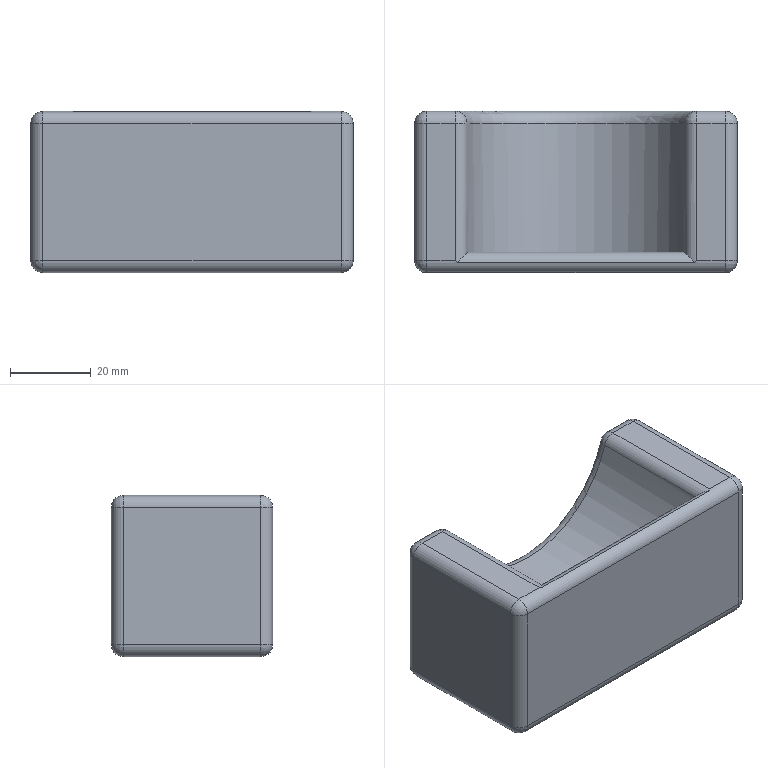Part | SolidWorks | features Extrusion 1, Fillet 1, ICE 1 | 1 solid | 36 faces | box 80 x 40 x 40 mm | volume 93219 mm3 | cylinder 17 | sphere 10 | plane 8 | torus 1 | commonest cylinder face diameters 6 x16 56 x1
STEP:
#1=CARTESIAN_POINT('',(29.95,3.,20.));
#2=VERTEX_POINT('',#1);
#3=CARTESIAN_POINT('',(37.,3.,20.));
#4=VERTEX_POINT('',#3);
#5=CARTESIAN_POINT('',(-40.,3.,20.));
#6=DIRECTION('',(1.,0.,0.));
#7=VECTOR('',#6,1000.);
#8=LINE('',#5,#7);
#9=EDGE_CURVE('',#2,#4,#8,.T.);
#10=ORIENTED_EDGE('',*,*,#9,.T.);
#11=CARTESIAN_POINT('',(37.,37.,20.));
#12=VERTEX_POINT('',#11);
#13=CARTESIAN_POINT('',(37.,40.,20.));
#14=DIRECTION('',(0.,1.,0.));
#15=VECTOR('',#14,1000.);
#16=LINE('',#13,#15);
#17=EDGE_CURVE('',#4,#12,#16,.T.);
#18=ORIENTED_EDGE('',*,*,#17,.T.);
#19=CARTESIAN_POINT('',(29.95,37.,20.));
#20=VERTEX_POINT('',#19);
#21=CARTESIAN_POINT('',(27.55,37.,20.));
#22=DIRECTION('',(-1.,0.,0.));
#23=VECTOR('',#22,1000.);
#24=LINE('',#21,#23);
#25=EDGE_CURVE('',#12,#20,#24,.T.);
#26=ORIENTED_EDGE('',*,*,#25,.T.);
#27=CARTESIAN_POINT('',(29.95,40.,20.));
#28=DIRECTION('',(0.,-1.,0.));
#29=VECTOR('',#28,1000.);
#30=LINE('',#27,#29);
#31=EDGE_CURVE('',#20,#2,#30,.T.);
#32=ORIENTED_EDGE('',*,*,#31,.T.);
#33=EDGE_LOOP('',(#10,#18,#26,#32));
#34=FACE_OUTER_BOUND('',#33,.T.);
#35=CARTESIAN_POINT('',(-40.,40.,20.));
#36=DIRECTION('',(0.,0.,-1.));
#37=DIRECTION('',(-1.,0.,0.));
#38=AXIS2_PLACEMENT_3D('',#35,#36,#37);
#39=PLANE('',#38);
#40=ADVANCED_FACE('',(#34),#39,.F.);
#41=CARTESIAN_POINT('',(40.,3.,-17.));
#42=VERTEX_POINT('',#41);
#43=CARTESIAN_POINT('',(40.,37.,-17.));
#44=VERTEX_POINT('',#43);
#45=CARTESIAN_POINT('',(40.,40.,-17.));
#46=DIRECTION('',(0.,1.,0.));
#47=VECTOR('',#46,1000.);
#48=LINE('',#45,#47);
#49=EDGE_CURVE('',#42,#44,#48,.T.);
#50=ORIENTED_EDGE('',*,*,#49,.T.);
#51=CARTESIAN_POINT('',(40.,37.,17.));
#52=VERTEX_POINT('',#51);
#53=CARTESIAN_POINT('',(40.,37.,20.));
#54=DIRECTION('',(0.,0.,1.));
#55=VECTOR('',#54,1000.);
#56=LINE('',#53,#55);
#57=EDGE_CURVE('',#44,#52,#56,.T.);
#58=ORIENTED_EDGE('',*,*,#57,.T.);
#59=CARTESIAN_POINT('',(40.,3.,17.));
#60=VERTEX_POINT('',#59);
#61=CARTESIAN_POINT('',(40.,40.,17.));
#62=DIRECTION('',(0.,-1.,0.));
#63=VECTOR('',#62,1000.);
#64=LINE('',#61,#63);
#65=EDGE_CURVE('',#52,#60,#64,.T.);
#66=ORIENTED_EDGE('',*,*,#65,.T.);
#67=CARTESIAN_POINT('',(40.,3.,-20.));
#68=DIRECTION('',(0.,0.,-1.));
#69=VECTOR('',#68,1000.);
#70=LINE('',#67,#69);
#71=EDGE_CURVE('',#60,#42,#70,.T.);
#72=ORIENTED_EDGE('',*,*,#71,.T.);
#73=EDGE_LOOP('',(#50,#58,#66,#72));
#74=FACE_OUTER_BOUND('',#73,.T.);
#75=CARTESIAN_POINT('',(40.,40.,-20.));
#76=DIRECTION('',(-1.,0.,0.));
#77=DIRECTION('',(0.,0.,1.));
#78=AXIS2_PLACEMENT_3D('',#75,#76,#77);
#79=PLANE('',#78);
#80=ADVANCED_FACE('',(#74),#79,.F.);
#81=CARTESIAN_POINT('',(-37.,37.,-20.));
#82=VERTEX_POINT('',#81);
#83=CARTESIAN_POINT('',(37.,37.,-20.));
#84=VERTEX_POINT('',#83);
#85=CARTESIAN_POINT('',(40.,37.,-20.));
#86=DIRECTION('',(1.,0.,0.));
#87=VECTOR('',#86,1000.);
#88=LINE('',#85,#87);
#89=EDGE_CURVE('',#82,#84,#88,.T.);
#90=ORIENTED_EDGE('',*,*,#89,.T.);
#91=CARTESIAN_POINT('',(37.,3.,-20.));
#92=VERTEX_POINT('',#91);
#93=CARTESIAN_POINT('',(37.,40.,-20.));
#94=DIRECTION('',(0.,-1.,0.));
#95=VECTOR('',#94,1000.);
#96=LINE('',#93,#95);
#97=EDGE_CURVE('',#84,#92,#96,.T.);
#98=ORIENTED_EDGE('',*,*,#97,.T.);
#99=CARTESIAN_POINT('',(-37.,3.,-20.));
#100=VERTEX_POINT('',#99);
#101=CARTESIAN_POINT('',(-40.,3.,-20.));
#102=DIRECTION('',(-1.,0.,0.));
#103=VECTOR('',#102,1000.);
#104=LINE('',#101,#103);
#105=EDGE_CURVE('',#92,#100,#104,.T.);
#106=ORIENTED_EDGE('',*,*,#105,.T.);
#107=CARTESIAN_POINT('',(-37.,40.,-20.));
#108=DIRECTION('',(0.,1.,0.));
#109=VECTOR('',#108,1000.);
#110=LINE('',#107,#109);
#111=EDGE_CURVE('',#100,#82,#110,.T.);
#112=ORIENTED_EDGE('',*,*,#111,.T.);
#113=EDGE_LOOP('',(#90,#98,#106,#112));
#114=FACE_OUTER_BOUND('',#113,.T.);
#115=CARTESIAN_POINT('',(-40.,40.,-20.));
#116=DIRECTION('',(0.,0.,1.));
#117=DIRECTION('',(1.,0.,0.));
#118=AXIS2_PLACEMENT_3D('',#115,#116,#117);
#119=PLANE('',#118);
#120=ADVANCED_FACE('',(#114),#119,.F.);
#121=CARTESIAN_POINT('',(-40.,37.,17.));
#122=VERTEX_POINT('',#121);
#123=CARTESIAN_POINT('',(-40.,37.,-17.));
#124=VERTEX_POINT('',#123);
#125=CARTESIAN_POINT('',(-40.,37.,-20.));
#126=DIRECTION('',(0.,0.,-1.));
#127=VECTOR('',#126,1000.);
#128=LINE('',#125,#127);
#129=EDGE_CURVE('',#122,#124,#128,.T.);
#130=ORIENTED_EDGE('',*,*,#129,.T.);
#131=CARTESIAN_POINT('',(-40.,3.,-17.));
#132=VERTEX_POINT('',#131);
#133=CARTESIAN_POINT('',(-40.,40.,-17.));
#134=DIRECTION('',(0.,-1.,0.));
#135=VECTOR('',#134,1000.);
#136=LINE('',#133,#135);
#137=EDGE_CURVE('',#124,#132,#136,.T.);
#138=ORIENTED_EDGE('',*,*,#137,.T.);
#139=CARTESIAN_POINT('',(-40.,3.,17.));
#140=VERTEX_POINT('',#139);
#141=CARTESIAN_POINT('',(-40.,3.,-20.));
#142=DIRECTION('',(0.,0.,1.));
#143=VECTOR('',#142,1000.);
#144=LINE('',#141,#143);
#145=EDGE_CURVE('',#132,#140,#144,.T.);
#146=ORIENTED_EDGE('',*,*,#145,.T.);
#147=CARTESIAN_POINT('',(-40.,40.,17.));
#148=DIRECTION('',(0.,1.,0.));
#149=VECTOR('',#148,1000.);
#150=LINE('',#147,#149);
#151=EDGE_CURVE('',#140,#122,#150,.T.);
#152=ORIENTED_EDGE('',*,*,#151,.T.);
#153=EDGE_LOOP('',(#130,#138,#146,#152));
#154=FACE_OUTER_BOUND('',#153,.T.);
#155=CARTESIAN_POINT('',(-40.,40.,-20.));
#156=DIRECTION('',(1.,0.,0.));
#157=DIRECTION('',(0.,0.,-1.));
#158=AXIS2_PLACEMENT_3D('',#155,#156,#157);
#159=PLANE('',#158);
#160=ADVANCED_FACE('',(#154),#159,.F.);
#161=CARTESIAN_POINT('',(-29.95,3.,20.));
#162=VERTEX_POINT('',#161);
#163=CARTESIAN_POINT('',(-29.95,37.,20.));
#164=VERTEX_POINT('',#163);
#165=CARTESIAN_POINT('',(-29.95,40.,20.));
#166=DIRECTION('',(0.,1.,0.));
#167=VECTOR('',#166,1000.);
#168=LINE('',#165,#167);
#169=EDGE_CURVE('',#162,#164,#168,.T.);
#170=ORIENTED_EDGE('',*,*,#169,.T.);
#171=CARTESIAN_POINT('',(-37.,37.,20.));
#172=VERTEX_POINT('',#171);
#173=CARTESIAN_POINT('',(-40.,37.,20.));
#174=DIRECTION('',(-1.,0.,0.));
#175=VECTOR('',#174,1000.);
#176=LINE('',#173,#175);
#177=EDGE_CURVE('',#164,#172,#176,.T.);
#178=ORIENTED_EDGE('',*,*,#177,.T.);
#179=CARTESIAN_POINT('',(-37.,3.,20.));
#180=VERTEX_POINT('',#179);
#181=CARTESIAN_POINT('',(-37.,40.,20.));
#182=DIRECTION('',(0.,-1.,0.));
#183=VECTOR('',#182,1000.);
#184=LINE('',#181,#183);
#185=EDGE_CURVE('',#172,#180,#184,.T.);
#186=ORIENTED_EDGE('',*,*,#185,.T.);
#187=CARTESIAN_POINT('',(-40.,3.,20.));
#188=DIRECTION('',(1.,0.,0.));
#189=VECTOR('',#188,1000.);
#190=LINE('',#187,#189);
#191=EDGE_CURVE('',#180,#162,#190,.T.);
#192=ORIENTED_EDGE('',*,*,#191,.T.);
#193=EDGE_LOOP('',(#170,#178,#186,#192));
#194=FACE_OUTER_BOUND('',#193,.T.);
#195=CARTESIAN_POINT('',(-40.,40.,20.));
#196=DIRECTION('',(0.,0.,-1.));
#197=DIRECTION('',(-1.,0.,0.));
#198=AXIS2_PLACEMENT_3D('',#195,#196,#197);
#199=PLANE('',#198);
#200=ADVANCED_FACE('',(#194),#199,.F.);
#201=CARTESIAN_POINT('',(-29.95,40.,17.));
#202=VERTEX_POINT('',#201);
#203=CARTESIAN_POINT('',(29.95,40.,17.));
#204=VERTEX_POINT('',#203);
#205=CARTESIAN_POINT('',(0.,40.,25.));
#206=DIRECTION('',(0.,-1.,0.));
#207=DIRECTION('',(0.,0.,1.));
#208=AXIS2_PLACEMENT_3D('',#205,#206,#207);
#209=CIRCLE('',#208,31.);
#210=EDGE_CURVE('',#202,#204,#209,.T.);
#211=ORIENTED_EDGE('',*,*,#210,.T.);
#212=CARTESIAN_POINT('',(37.,40.,17.));
#213=VERTEX_POINT('',#212);
#214=CARTESIAN_POINT('',(40.,40.,17.));
#215=DIRECTION('',(1.,0.,0.));
#216=VECTOR('',#215,1000.);
#217=LINE('',#214,#216);
#218=EDGE_CURVE('',#204,#213,#217,.T.);
#219=ORIENTED_EDGE('',*,*,#218,.T.);
#220=CARTESIAN_POINT('',(37.,40.,-17.));
#221=VERTEX_POINT('',#220);
#222=CARTESIAN_POINT('',(37.,40.,-20.));
#223=DIRECTION('',(0.,0.,-1.));
#224=VECTOR('',#223,1000.);
#225=LINE('',#222,#224);
#226=EDGE_CURVE('',#213,#221,#225,.T.);
#227=ORIENTED_EDGE('',*,*,#226,.T.);
#228=CARTESIAN_POINT('',(-37.,40.,-17.));
#229=VERTEX_POINT('',#228);
#230=CARTESIAN_POINT('',(-40.,40.,-17.));
#231=DIRECTION('',(-1.,0.,0.));
#232=VECTOR('',#231,1000.);
#233=LINE('',#230,#232);
#234=EDGE_CURVE('',#221,#229,#233,.T.);
#235=ORIENTED_EDGE('',*,*,#234,.T.);
#236=CARTESIAN_POINT('',(-37.,40.,17.));
#237=VERTEX_POINT('',#236);
#238=CARTESIAN_POINT('',(-37.,40.,20.));
#239=DIRECTION('',(0.,0.,1.));
#240=VECTOR('',#239,1000.);
#241=LINE('',#238,#240);
#242=EDGE_CURVE('',#229,#237,#241,.T.);
#243=ORIENTED_EDGE('',*,*,#242,.T.);
#244=CARTESIAN_POINT('',(-27.55,40.,17.));
#245=DIRECTION('',(1.,0.,0.));
#246=VECTOR('',#245,1000.);
#247=LINE('',#244,#246);
#248=EDGE_CURVE('',#237,#202,#247,.T.);
#249=ORIENTED_EDGE('',*,*,#248,.T.);
#250=EDGE_LOOP('',(#211,#219,#227,#235,#243,#249));
#251=FACE_OUTER_BOUND('',#250,.T.);
#252=CARTESIAN_POINT('',(0.,40.,0.));
#253=DIRECTION('',(0.,1.,0.));
#254=DIRECTION('',(0.,0.,1.));
#255=AXIS2_PLACEMENT_3D('',#252,#253,#254);
#256=PLANE('',#255);
#257=ADVANCED_FACE('',(#251),#256,.T.);
#258=CARTESIAN_POINT('',(-37.,0.,17.));
#259=VERTEX_POINT('',#258);
#260=CARTESIAN_POINT('',(-37.,0.,-17.));
#261=VERTEX_POINT('',#260);
#262=CARTESIAN_POINT('',(-37.,0.,0.));
#263=DIRECTION('',(0.,0.,-1.));
#264=VECTOR('',#263,1000.);
#265=LINE('',#262,#264);
#266=EDGE_CURVE('',#259,#261,#265,.T.);
#267=ORIENTED_EDGE('',*,*,#266,.T.);
#268=CARTESIAN_POINT('',(37.,0.,-17.));
#269=VERTEX_POINT('',#268);
#270=CARTESIAN_POINT('',(0.,0.,-17.));
#271=DIRECTION('',(1.,0.,0.));
#272=VECTOR('',#271,1000.);
#273=LINE('',#270,#272);
#274=EDGE_CURVE('',#261,#269,#273,.T.);
#275=ORIENTED_EDGE('',*,*,#274,.T.);
#276=CARTESIAN_POINT('',(37.,0.,17.));
#277=VERTEX_POINT('',#276);
#278=CARTESIAN_POINT('',(37.,0.,0.));
#279=DIRECTION('',(0.,0.,1.));
#280=VECTOR('',#279,1000.);
#281=LINE('',#278,#280);
#282=EDGE_CURVE('',#269,#277,#281,.T.);
#283=ORIENTED_EDGE('',*,*,#282,.T.);
#284=CARTESIAN_POINT('',(0.,0.,17.));
#285=DIRECTION('',(-1.,0.,0.));
#286=VECTOR('',#285,1000.);
#287=LINE('',#284,#286);
#288=EDGE_CURVE('',#277,#259,#287,.T.);
#289=ORIENTED_EDGE('',*,*,#288,.T.);
#290=EDGE_LOOP('',(#267,#275,#283,#289));
#291=FACE_OUTER_BOUND('',#290,.T.);
#292=CARTESIAN_POINT('',(0.,0.,0.));
#293=DIRECTION('',(0.,1.,0.));
#294=DIRECTION('',(0.,0.,1.));
#295=AXIS2_PLACEMENT_3D('',#292,#293,#294);
#296=PLANE('',#295);
#297=ADVANCED_FACE('',(#291),#296,.F.);
#298=CARTESIAN_POINT('',(26.833,5.,17.));
#299=VERTEX_POINT('',#298);
#300=CARTESIAN_POINT('',(-26.833,5.,17.));
#301=VERTEX_POINT('',#300);
#302=CARTESIAN_POINT('',(0.,5.,25.));
#303=DIRECTION('',(0.,1.,0.));
#304=DIRECTION('',(0.,0.,1.));
#305=AXIS2_PLACEMENT_3D('',#302,#303,#304);
#306=CIRCLE('',#305,28.);
#307=EDGE_CURVE('',#299,#301,#306,.T.);
#308=ORIENTED_EDGE('',*,*,#307,.T.);
#309=CARTESIAN_POINT('',(27.55,5.,17.));
#310=DIRECTION('',(1.,0.,0.));
#311=VECTOR('',#310,1000.);
#312=LINE('',#309,#311);
#313=EDGE_CURVE('',#301,#299,#312,.T.);
#314=ORIENTED_EDGE('',*,*,#313,.T.);
#315=EDGE_LOOP('',(#308,#314));
#316=FACE_OUTER_BOUND('',#315,.T.);
#317=CARTESIAN_POINT('',(0.,5.,25.));
#318=DIRECTION('',(0.,1.,0.));
#319=DIRECTION('',(0.,0.,1.));
#320=AXIS2_PLACEMENT_3D('',#317,#318,#319);
#321=PLANE('',#320);
#322=ADVANCED_FACE('',(#316),#321,.T.);
#323=ORIENTED_EDGE('',*,*,#307,.F.);
#324=CARTESIAN_POINT('',(27.052,4.898,17.774));
#325=VERTEX_POINT('',#324);
#326=CARTESIAN_POINT('',(26.833,5.,17.));
#327=CARTESIAN_POINT('',(26.911,5.,17.261));
#328=CARTESIAN_POINT('',(26.983,4.966,17.519));
#329=CARTESIAN_POINT('',(27.052,4.898,17.774));
#330=B_SPLINE_CURVE_WITH_KNOTS('',3,(#326,#327,#328,#329),.UNSPECIFIED.,.F.,.F.,(4,4),(0.,0.0008109),.UNSPECIFIED.);
#331=EDGE_CURVE('',#299,#325,#330,.T.);
#332=ORIENTED_EDGE('',*,*,#331,.T.);
#333=CARTESIAN_POINT('',(27.052,37.,17.774));
#334=VERTEX_POINT('',#333);
#335=CARTESIAN_POINT('',(27.052,5.,17.774));
#336=DIRECTION('',(0.,1.,0.));
#337=VECTOR('',#336,1000.);
#338=LINE('',#335,#337);
#339=EDGE_CURVE('',#325,#334,#338,.T.);
#340=ORIENTED_EDGE('',*,*,#339,.T.);
#341=CARTESIAN_POINT('',(-27.052,37.,17.774));
#342=VERTEX_POINT('',#341);
#343=CARTESIAN_POINT('',(0.,37.,25.));
#344=DIRECTION('',(0.,1.,0.));
#345=DIRECTION('',(0.,0.,1.));
#346=AXIS2_PLACEMENT_3D('',#343,#344,#345);
#347=CIRCLE('',#346,28.);
#348=EDGE_CURVE('',#334,#342,#347,.T.);
#349=ORIENTED_EDGE('',*,*,#348,.T.);
#350=CARTESIAN_POINT('',(-27.052,4.898,17.774));
#351=VERTEX_POINT('',#350);
#352=CARTESIAN_POINT('',(-27.052,5.,17.774));
#353=DIRECTION('',(0.,-1.,0.));
#354=VECTOR('',#353,1000.);
#355=LINE('',#352,#354);
#356=EDGE_CURVE('',#342,#351,#355,.T.);
#357=ORIENTED_EDGE('',*,*,#356,.T.);
#358=CARTESIAN_POINT('',(-27.052,4.898,17.774));
#359=CARTESIAN_POINT('',(-26.983,4.966,17.519));
#360=CARTESIAN_POINT('',(-26.911,5.,17.261));
#361=CARTESIAN_POINT('',(-26.833,5.,17.));
#362=B_SPLINE_CURVE_WITH_KNOTS('',3,(#358,#359,#360,#361),.UNSPECIFIED.,.F.,.F.,(4,4),(0.,0.0008109),.UNSPECIFIED.);
#363=EDGE_CURVE('',#351,#301,#362,.T.);
#364=ORIENTED_EDGE('',*,*,#363,.T.);
#365=EDGE_LOOP('',(#323,#332,#340,#349,#357,#364));
#366=FACE_OUTER_BOUND('',#365,.T.);
#367=CARTESIAN_POINT('',(0.,5.,25.));
#368=DIRECTION('',(0.,1.,0.));
#369=DIRECTION('',(0.,0.,1.));
#370=AXIS2_PLACEMENT_3D('',#367,#368,#369);
#371=CYLINDRICAL_SURFACE('',#370,28.);
#372=ADVANCED_FACE('',(#366),#371,.F.);
#373=CARTESIAN_POINT('',(-37.,3.,-17.));
#374=DIRECTION('',(-1.,0.,0.));
#375=DIRECTION('',(0.,0.,1.));
#376=AXIS2_PLACEMENT_3D('',#373,#374,#375);
#377=CIRCLE('',#376,3.);
#378=EDGE_CURVE('',#100,#261,#377,.T.);
#379=ORIENTED_EDGE('',*,*,#378,.F.);
#380=ORIENTED_EDGE('',*,*,#105,.F.);
#381=CARTESIAN_POINT('',(37.,3.,-17.));
#382=DIRECTION('',(1.,0.,0.));
#383=DIRECTION('',(0.,0.,-1.));
#384=AXIS2_PLACEMENT_3D('',#381,#382,#383);
#385=CIRCLE('',#384,3.);
#386=EDGE_CURVE('',#269,#92,#385,.T.);
#387=ORIENTED_EDGE('',*,*,#386,.F.);
#388=ORIENTED_EDGE('',*,*,#274,.F.);
#389=EDGE_LOOP('',(#379,#380,#387,#388));
#390=FACE_OUTER_BOUND('',#389,.T.);
#391=CARTESIAN_POINT('',(-40.,3.,-17.));
#392=DIRECTION('',(-1.,0.,0.));
#393=DIRECTION('',(0.,0.,1.));
#394=AXIS2_PLACEMENT_3D('',#391,#392,#393);
#395=CYLINDRICAL_SURFACE('',#394,3.);
#396=ADVANCED_FACE('',(#390),#395,.T.);
#397=CARTESIAN_POINT('',(37.,37.,-17.));
#398=DIRECTION('',(0.,1.,0.));
#399=DIRECTION('',(0.,0.,1.));
#400=AXIS2_PLACEMENT_3D('',#397,#398,#399);
#401=CIRCLE('',#400,3.);
#402=EDGE_CURVE('',#44,#84,#401,.T.);
#403=ORIENTED_EDGE('',*,*,#402,.F.);
#404=ORIENTED_EDGE('',*,*,#49,.F.);
#405=CARTESIAN_POINT('',(37.,3.,-17.));
#406=DIRECTION('',(0.,-1.,0.));
#407=DIRECTION('',(0.,0.,-1.));
#408=AXIS2_PLACEMENT_3D('',#405,#406,#407);
#409=CIRCLE('',#408,3.);
#410=EDGE_CURVE('',#92,#42,#409,.T.);
#411=ORIENTED_EDGE('',*,*,#410,.F.);
#412=ORIENTED_EDGE('',*,*,#97,.F.);
#413=EDGE_LOOP('',(#403,#404,#411,#412));
#414=FACE_OUTER_BOUND('',#413,.T.);
#415=CARTESIAN_POINT('',(37.,40.,-17.));
#416=DIRECTION('',(0.,-1.,0.));
#417=DIRECTION('',(0.,0.,-1.));
#418=AXIS2_PLACEMENT_3D('',#415,#416,#417);
#419=CYLINDRICAL_SURFACE('',#418,3.);
#420=ADVANCED_FACE('',(#414),#419,.T.);
#421=CARTESIAN_POINT('',(37.,37.,17.));
#422=DIRECTION('',(0.,0.,1.));
#423=DIRECTION('',(0.,-1.,0.));
#424=AXIS2_PLACEMENT_3D('',#421,#422,#423);
#425=CIRCLE('',#424,3.);
#426=EDGE_CURVE('',#52,#213,#425,.T.);
#427=ORIENTED_EDGE('',*,*,#426,.F.);
#428=ORIENTED_EDGE('',*,*,#57,.F.);
#429=CARTESIAN_POINT('',(37.,37.,-17.));
#430=DIRECTION('',(0.,0.,-1.));
#431=DIRECTION('',(-1.,0.,0.));
#432=AXIS2_PLACEMENT_3D('',#429,#430,#431);
#433=CIRCLE('',#432,3.);
#434=EDGE_CURVE('',#221,#44,#433,.T.);
#435=ORIENTED_EDGE('',*,*,#434,.F.);
#436=ORIENTED_EDGE('',*,*,#226,.F.);
#437=EDGE_LOOP('',(#427,#428,#435,#436));
#438=FACE_OUTER_BOUND('',#437,.T.);
#439=CARTESIAN_POINT('',(37.,37.,0.));
#440=DIRECTION('',(0.,0.,1.));
#441=DIRECTION('',(1.,0.,0.));
#442=AXIS2_PLACEMENT_3D('',#439,#440,#441);
#443=CYLINDRICAL_SURFACE('',#442,3.);
#444=ADVANCED_FACE('',(#438),#443,.T.);
#445=ORIENTED_EDGE('',*,*,#386,.T.);
#446=ORIENTED_EDGE('',*,*,#410,.T.);
#447=CARTESIAN_POINT('',(37.,3.,-17.));
#448=DIRECTION('',(0.,0.,1.));
#449=DIRECTION('',(-1.,0.,0.));
#450=AXIS2_PLACEMENT_3D('',#447,#448,#449);
#451=CIRCLE('',#450,3.);
#452=EDGE_CURVE('',#269,#42,#451,.T.);
#453=ORIENTED_EDGE('',*,*,#452,.F.);
#454=EDGE_LOOP('',(#445,#446,#453));
#455=FACE_OUTER_BOUND('',#454,.T.);
#456=CARTESIAN_POINT('',(37.,3.,-17.));
#457=DIRECTION('',(0.,1.,0.));
#458=DIRECTION('',(1.,0.,0.));
#459=AXIS2_PLACEMENT_3D('',#456,#457,#458);
#460=SPHERICAL_SURFACE('',#459,3.);
#461=ADVANCED_FACE('',(#455),#460,.T.);
#462=CARTESIAN_POINT('',(-37.,3.,-17.));
#463=DIRECTION('',(0.,1.,0.));
#464=DIRECTION('',(0.,0.,-1.));
#465=AXIS2_PLACEMENT_3D('',#462,#463,#464);
#466=CIRCLE('',#465,3.);
#467=EDGE_CURVE('',#100,#132,#466,.T.);
#468=ORIENTED_EDGE('',*,*,#467,.F.);
#469=ORIENTED_EDGE('',*,*,#378,.T.);
#470=CARTESIAN_POINT('',(-37.,3.,-17.));
#471=DIRECTION('',(0.,0.,1.));
#472=DIRECTION('',(-1.,0.,0.));
#473=AXIS2_PLACEMENT_3D('',#470,#471,#472);
#474=CIRCLE('',#473,3.);
#475=EDGE_CURVE('',#132,#261,#474,.T.);
#476=ORIENTED_EDGE('',*,*,#475,.F.);
#477=EDGE_LOOP('',(#468,#469,#476));
#478=FACE_OUTER_BOUND('',#477,.T.);
#479=CARTESIAN_POINT('',(-37.,3.,-17.));
#480=DIRECTION('',(0.,1.,0.));
#481=DIRECTION('',(1.,0.,0.));
#482=AXIS2_PLACEMENT_3D('',#479,#480,#481);
#483=SPHERICAL_SURFACE('',#482,3.);
#484=ADVANCED_FACE('',(#478),#483,.T.);
#485=ORIENTED_EDGE('',*,*,#434,.T.);
#486=ORIENTED_EDGE('',*,*,#402,.T.);
#487=CARTESIAN_POINT('',(37.,37.,-17.));
#488=DIRECTION('',(-1.,0.,0.));
#489=DIRECTION('',(0.,0.,-1.));
#490=AXIS2_PLACEMENT_3D('',#487,#488,#489);
#491=CIRCLE('',#490,3.);
#492=EDGE_CURVE('',#221,#84,#491,.T.);
#493=ORIENTED_EDGE('',*,*,#492,.F.);
#494=EDGE_LOOP('',(#485,#486,#493));
#495=FACE_OUTER_BOUND('',#494,.T.);
#496=CARTESIAN_POINT('',(37.,37.,-17.));
#497=DIRECTION('',(0.,1.,0.));
#498=DIRECTION('',(1.,0.,0.));
#499=AXIS2_PLACEMENT_3D('',#496,#497,#498);
#500=SPHERICAL_SURFACE('',#499,3.);
#501=ADVANCED_FACE('',(#495),#500,.T.);
#502=CARTESIAN_POINT('',(37.,37.,17.));
#503=DIRECTION('',(-1.,0.,0.));
#504=DIRECTION('',(0.,0.,-1.));
#505=AXIS2_PLACEMENT_3D('',#502,#503,#504);
#506=CIRCLE('',#505,3.);
#507=EDGE_CURVE('',#12,#213,#506,.T.);
#508=ORIENTED_EDGE('',*,*,#507,.F.);
#509=CARTESIAN_POINT('',(37.,37.,17.));
#510=DIRECTION('',(0.,-1.,0.));
#511=DIRECTION('',(0.,0.,1.));
#512=AXIS2_PLACEMENT_3D('',#509,#510,#511);
#513=CIRCLE('',#512,3.);
#514=EDGE_CURVE('',#52,#12,#513,.T.);
#515=ORIENTED_EDGE('',*,*,#514,.F.);
#516=ORIENTED_EDGE('',*,*,#426,.T.);
#517=EDGE_LOOP('',(#508,#515,#516));
#518=FACE_OUTER_BOUND('',#517,.T.);
#519=CARTESIAN_POINT('',(37.,37.,17.));
#520=DIRECTION('',(0.,1.,0.));
#521=DIRECTION('',(1.,0.,0.));
#522=AXIS2_PLACEMENT_3D('',#519,#520,#521);
#523=SPHERICAL_SURFACE('',#522,3.);
#524=ADVANCED_FACE('',(#518),#523,.T.);
#525=ORIENTED_EDGE('',*,*,#514,.T.);
#526=ORIENTED_EDGE('',*,*,#17,.F.);
#527=CARTESIAN_POINT('',(37.,3.,17.));
#528=DIRECTION('',(0.,-1.,0.));
#529=DIRECTION('',(0.,0.,-1.));
#530=AXIS2_PLACEMENT_3D('',#527,#528,#529);
#531=CIRCLE('',#530,3.);
#532=EDGE_CURVE('',#60,#4,#531,.T.);
#533=ORIENTED_EDGE('',*,*,#532,.F.);
#534=ORIENTED_EDGE('',*,*,#65,.F.);
#535=EDGE_LOOP('',(#525,#526,#533,#534));
#536=FACE_OUTER_BOUND('',#535,.T.);
#537=CARTESIAN_POINT('',(37.,40.,17.));
#538=DIRECTION('',(0.,-1.,0.));
#539=DIRECTION('',(0.,0.,-1.));
#540=AXIS2_PLACEMENT_3D('',#537,#538,#539);
#541=CYLINDRICAL_SURFACE('',#540,3.);
#542=ADVANCED_FACE('',(#536),#541,.T.);
#543=ORIENTED_EDGE('',*,*,#452,.T.);
#544=ORIENTED_EDGE('',*,*,#71,.F.);
#545=CARTESIAN_POINT('',(37.,3.,17.));
#546=DIRECTION('',(0.,0.,1.));
#547=DIRECTION('',(1.,0.,0.));
#548=AXIS2_PLACEMENT_3D('',#545,#546,#547);
#549=CIRCLE('',#548,3.);
#550=EDGE_CURVE('',#277,#60,#549,.T.);
#551=ORIENTED_EDGE('',*,*,#550,.F.);
#552=ORIENTED_EDGE('',*,*,#282,.F.);
#553=EDGE_LOOP('',(#543,#544,#551,#552));
#554=FACE_OUTER_BOUND('',#553,.T.);
#555=CARTESIAN_POINT('',(37.,3.,-20.));
#556=DIRECTION('',(0.,0.,-1.));
#557=DIRECTION('',(-1.,0.,0.));
#558=AXIS2_PLACEMENT_3D('',#555,#556,#557);
#559=CYLINDRICAL_SURFACE('',#558,3.);
#560=ADVANCED_FACE('',(#554),#559,.T.);
#561=ORIENTED_EDGE('',*,*,#475,.T.);
#562=ORIENTED_EDGE('',*,*,#266,.F.);
#563=CARTESIAN_POINT('',(-37.,3.,17.));
#564=DIRECTION('',(0.,0.,1.));
#565=DIRECTION('',(1.,0.,0.));
#566=AXIS2_PLACEMENT_3D('',#563,#564,#565);
#567=CIRCLE('',#566,3.);
#568=EDGE_CURVE('',#140,#259,#567,.T.);
#569=ORIENTED_EDGE('',*,*,#568,.F.);
#570=ORIENTED_EDGE('',*,*,#145,.F.);
#571=EDGE_LOOP('',(#561,#562,#569,#570));
#572=FACE_OUTER_BOUND('',#571,.T.);
#573=CARTESIAN_POINT('',(-37.,3.,-20.));
#574=DIRECTION('',(0.,0.,1.));
#575=DIRECTION('',(1.,0.,0.));
#576=AXIS2_PLACEMENT_3D('',#573,#574,#575);
#577=CYLINDRICAL_SURFACE('',#576,3.);
#578=ADVANCED_FACE('',(#572),#577,.T.);
#579=ORIENTED_EDGE('',*,*,#467,.T.);
#580=ORIENTED_EDGE('',*,*,#137,.F.);
#581=CARTESIAN_POINT('',(-37.,37.,-17.));
#582=DIRECTION('',(0.,1.,0.));
#583=DIRECTION('',(0.,0.,1.));
#584=AXIS2_PLACEMENT_3D('',#581,#582,#583);
#585=CIRCLE('',#584,3.);
#586=EDGE_CURVE('',#82,#124,#585,.T.);
#587=ORIENTED_EDGE('',*,*,#586,.F.);
#588=ORIENTED_EDGE('',*,*,#111,.F.);
#589=EDGE_LOOP('',(#579,#580,#587,#588));
#590=FACE_OUTER_BOUND('',#589,.T.);
#591=CARTESIAN_POINT('',(-37.,40.,-17.));
#592=DIRECTION('',(0.,-1.,0.));
#593=DIRECTION('',(0.,0.,-1.));
#594=AXIS2_PLACEMENT_3D('',#591,#592,#593);
#595=CYLINDRICAL_SURFACE('',#594,3.);
#596=ADVANCED_FACE('',(#590),#595,.T.);
#597=ORIENTED_EDGE('',*,*,#492,.T.);
#598=ORIENTED_EDGE('',*,*,#89,.F.);
#599=CARTESIAN_POINT('',(-37.,37.,-17.));
#600=DIRECTION('',(-1.,0.,0.));
#601=DIRECTION('',(0.,0.,1.));
#602=AXIS2_PLACEMENT_3D('',#599,#600,#601);
#603=CIRCLE('',#602,3.);
#604=EDGE_CURVE('',#229,#82,#603,.T.);
#605=ORIENTED_EDGE('',*,*,#604,.F.);
#606=ORIENTED_EDGE('',*,*,#234,.F.);
#607=EDGE_LOOP('',(#597,#598,#605,#606));
#608=FACE_OUTER_BOUND('',#607,.T.);
#609=CARTESIAN_POINT('',(0.,37.,-17.));
#610=DIRECTION('',(1.,0.,0.));
#611=DIRECTION('',(0.,0.,-1.));
#612=AXIS2_PLACEMENT_3D('',#609,#610,#611);
#613=CYLINDRICAL_SURFACE('',#612,3.);
#614=ADVANCED_FACE('',(#608),#613,.T.);
#615=ORIENTED_EDGE('',*,*,#507,.T.);
#616=ORIENTED_EDGE('',*,*,#218,.F.);
#617=CARTESIAN_POINT('',(29.95,37.,17.));
#618=DIRECTION('',(-1.,0.,0.));
#619=DIRECTION('',(0.,-1.,0.));
#620=AXIS2_PLACEMENT_3D('',#617,#618,#619);
#621=CIRCLE('',#620,3.);
#622=EDGE_CURVE('',#20,#204,#621,.T.);
#623=ORIENTED_EDGE('',*,*,#622,.F.);
#624=ORIENTED_EDGE('',*,*,#25,.F.);
#625=EDGE_LOOP('',(#615,#616,#623,#624));
#626=FACE_OUTER_BOUND('',#625,.T.);
#627=CARTESIAN_POINT('',(0.,37.,17.));
#628=DIRECTION('',(-1.,0.,0.));
#629=DIRECTION('',(0.,0.,1.));
#630=AXIS2_PLACEMENT_3D('',#627,#628,#629);
#631=CYLINDRICAL_SURFACE('',#630,3.);
#632=ADVANCED_FACE('',(#626),#631,.T.);
#633=CARTESIAN_POINT('',(29.45,2.5,19.958));
#634=VERTEX_POINT('',#633);
#635=CARTESIAN_POINT('',(29.95,3.,20.));
#636=CARTESIAN_POINT('',(29.782,2.832,20.));
#637=CARTESIAN_POINT('',(29.615,2.665,19.986));
#638=CARTESIAN_POINT('',(29.45,2.5,19.958));
#639=(BOUNDED_CURVE()B_SPLINE_CURVE(3,(#635,#636,#637,#638),.UNSPECIFIED.,.F.,.F.)B_SPLINE_CURVE_WITH_KNOTS((4,4),(1.571,1.738),.UNSPECIFIED.)CURVE()GEOMETRIC_REPRESENTATION_ITEM()RATIONAL_B_SPLINE_CURVE((1.,0.9977,0.9977,1.))REPRESENTATION_ITEM(''));
#640=EDGE_CURVE('',#2,#634,#639,.T.);
#641=ORIENTED_EDGE('',*,*,#640,.F.);
#642=ORIENTED_EDGE('',*,*,#31,.F.);
#643=CARTESIAN_POINT('',(29.95,37.,17.));
#644=DIRECTION('',(0.,1.,0.));
#645=DIRECTION('',(0.,0.,1.));
#646=AXIS2_PLACEMENT_3D('',#643,#644,#645);
#647=CIRCLE('',#646,3.);
#648=EDGE_CURVE('',#334,#20,#647,.T.);
#649=ORIENTED_EDGE('',*,*,#648,.F.);
#650=ORIENTED_EDGE('',*,*,#339,.F.);
#651=CARTESIAN_POINT('',(29.45,2.5,19.958));
#652=CARTESIAN_POINT('',(28.258,3.692,19.757));
#653=CARTESIAN_POINT('',(27.364,4.586,18.942));
#654=CARTESIAN_POINT('',(27.052,4.898,17.774));
#655=(BOUNDED_CURVE()B_SPLINE_CURVE(3,(#651,#652,#653,#654),.UNSPECIFIED.,.F.,.F.)B_SPLINE_CURVE_WITH_KNOTS((4,4),(4.88,6.022),.UNSPECIFIED.)CURVE()GEOMETRIC_REPRESENTATION_ITEM()RATIONAL_B_SPLINE_CURVE((1.,0.8942,0.8942,1.))REPRESENTATION_ITEM(''));
#656=EDGE_CURVE('',#634,#325,#655,.T.);
#657=ORIENTED_EDGE('',*,*,#656,.F.);
#658=EDGE_LOOP('',(#641,#642,#649,#650,#657));
#659=FACE_OUTER_BOUND('',#658,.T.);
#660=CARTESIAN_POINT('',(29.95,5.,17.));
#661=DIRECTION('',(0.,1.,0.));
#662=DIRECTION('',(0.,0.,1.));
#663=AXIS2_PLACEMENT_3D('',#660,#661,#662);
#664=CYLINDRICAL_SURFACE('',#663,3.);
#665=ADVANCED_FACE('',(#659),#664,.T.);
#666=ORIENTED_EDGE('',*,*,#550,.T.);
#667=ORIENTED_EDGE('',*,*,#532,.T.);
#668=CARTESIAN_POINT('',(37.,3.,17.));
#669=DIRECTION('',(-1.,0.,0.));
#670=DIRECTION('',(0.,0.,-1.));
#671=AXIS2_PLACEMENT_3D('',#668,#669,#670);
#672=CIRCLE('',#671,3.);
#673=EDGE_CURVE('',#277,#4,#672,.T.);
#674=ORIENTED_EDGE('',*,*,#673,.F.);
#675=EDGE_LOOP('',(#666,#667,#674));
#676=FACE_OUTER_BOUND('',#675,.T.);
#677=CARTESIAN_POINT('',(37.,3.,17.));
#678=DIRECTION('',(0.,1.,0.));
#679=DIRECTION('',(1.,0.,0.));
#680=AXIS2_PLACEMENT_3D('',#677,#678,#679);
#681=SPHERICAL_SURFACE('',#680,3.);
#682=ADVANCED_FACE('',(#676),#681,.T.);
#683=CARTESIAN_POINT('',(-37.,3.,17.));
#684=DIRECTION('',(0.,1.,0.));
#685=DIRECTION('',(0.,0.,-1.));
#686=AXIS2_PLACEMENT_3D('',#683,#684,#685);
#687=CIRCLE('',#686,3.);
#688=EDGE_CURVE('',#140,#180,#687,.T.);
#689=ORIENTED_EDGE('',*,*,#688,.F.);
#690=ORIENTED_EDGE('',*,*,#568,.T.);
#691=CARTESIAN_POINT('',(-37.,3.,17.));
#692=DIRECTION('',(1.,0.,0.));
#693=DIRECTION('',(0.,0.,1.));
#694=AXIS2_PLACEMENT_3D('',#691,#692,#693);
#695=CIRCLE('',#694,3.);
#696=EDGE_CURVE('',#180,#259,#695,.T.);
#697=ORIENTED_EDGE('',*,*,#696,.F.);
#698=EDGE_LOOP('',(#689,#690,#697));
#699=FACE_OUTER_BOUND('',#698,.T.);
#700=CARTESIAN_POINT('',(-37.,3.,17.));
#701=DIRECTION('',(0.,1.,0.));
#702=DIRECTION('',(1.,0.,0.));
#703=AXIS2_PLACEMENT_3D('',#700,#701,#702);
#704=SPHERICAL_SURFACE('',#703,3.);
#705=ADVANCED_FACE('',(#699),#704,.T.);
#706=ORIENTED_EDGE('',*,*,#604,.T.);
#707=ORIENTED_EDGE('',*,*,#586,.T.);
#708=CARTESIAN_POINT('',(-37.,37.,-17.));
#709=DIRECTION('',(0.,0.,1.));
#710=DIRECTION('',(-1.,0.,0.));
#711=AXIS2_PLACEMENT_3D('',#708,#709,#710);
#712=CIRCLE('',#711,3.);
#713=EDGE_CURVE('',#229,#124,#712,.T.);
#714=ORIENTED_EDGE('',*,*,#713,.F.);
#715=EDGE_LOOP('',(#706,#707,#714));
#716=FACE_OUTER_BOUND('',#715,.T.);
#717=CARTESIAN_POINT('',(-37.,37.,-17.));
#718=DIRECTION('',(0.,1.,0.));
#719=DIRECTION('',(1.,0.,0.));
#720=AXIS2_PLACEMENT_3D('',#717,#718,#719);
#721=SPHERICAL_SURFACE('',#720,3.);
#722=ADVANCED_FACE('',(#716),#721,.T.);
#723=ORIENTED_EDGE('',*,*,#648,.T.);
#724=ORIENTED_EDGE('',*,*,#622,.T.);
#725=CARTESIAN_POINT('',(29.95,37.,17.));
#726=DIRECTION('',(-0.2581,0.,-0.9661));
#727=DIRECTION('',(0.9661,0.,-0.2581));
#728=AXIS2_PLACEMENT_3D('',#725,#726,#727);
#729=CIRCLE('',#728,3.);
#730=EDGE_CURVE('',#334,#204,#729,.T.);
#731=ORIENTED_EDGE('',*,*,#730,.F.);
#732=EDGE_LOOP('',(#723,#724,#731));
#733=FACE_OUTER_BOUND('',#732,.T.);
#734=CARTESIAN_POINT('',(29.95,37.,17.));
#735=DIRECTION('',(0.,1.,0.));
#736=DIRECTION('',(1.,0.,0.));
#737=AXIS2_PLACEMENT_3D('',#734,#735,#736);
#738=SPHERICAL_SURFACE('',#737,3.);
#739=ADVANCED_FACE('',(#733),#738,.T.);
#740=CARTESIAN_POINT('',(-29.45,2.5,19.958));
#741=VERTEX_POINT('',#740);
#742=CARTESIAN_POINT('',(0.,2.5,19.958));
#743=DIRECTION('',(-1.,0.,0.));
#744=VECTOR('',#743,1000.);
#745=LINE('',#742,#744);
#746=EDGE_CURVE('',#634,#741,#745,.T.);
#747=ORIENTED_EDGE('',*,*,#746,.F.);
#748=ORIENTED_EDGE('',*,*,#656,.T.);
#749=ORIENTED_EDGE('',*,*,#331,.F.);
#750=ORIENTED_EDGE('',*,*,#313,.F.);
#751=ORIENTED_EDGE('',*,*,#363,.F.);
#752=CARTESIAN_POINT('',(-29.45,2.5,19.958));
#753=CARTESIAN_POINT('',(-28.258,3.692,19.757));
#754=CARTESIAN_POINT('',(-27.364,4.586,18.942));
#755=CARTESIAN_POINT('',(-27.052,4.898,17.774));
#756=(BOUNDED_CURVE()B_SPLINE_CURVE(3,(#752,#753,#754,#755),.UNSPECIFIED.,.F.,.F.)B_SPLINE_CURVE_WITH_KNOTS((4,4),(4.88,6.022),.UNSPECIFIED.)CURVE()GEOMETRIC_REPRESENTATION_ITEM()RATIONAL_B_SPLINE_CURVE((1.,0.8942,0.8942,1.))REPRESENTATION_ITEM(''));
#757=EDGE_CURVE('',#741,#351,#756,.T.);
#758=ORIENTED_EDGE('',*,*,#757,.F.);
#759=EDGE_LOOP('',(#747,#748,#749,#750,#751,#758));
#760=FACE_OUTER_BOUND('',#759,.T.);
#761=CARTESIAN_POINT('',(0.,2.,17.));
#762=DIRECTION('',(-1.,0.,0.));
#763=DIRECTION('',(0.,0.,1.));
#764=AXIS2_PLACEMENT_3D('',#761,#762,#763);
#765=CYLINDRICAL_SURFACE('',#764,3.);
#766=ADVANCED_FACE('',(#760),#765,.T.);
#767=ORIENTED_EDGE('',*,*,#640,.T.);
#768=ORIENTED_EDGE('',*,*,#746,.T.);
#769=CARTESIAN_POINT('',(-29.95,3.,20.));
#770=CARTESIAN_POINT('',(-29.782,2.832,20.));
#771=CARTESIAN_POINT('',(-29.615,2.665,19.986));
#772=CARTESIAN_POINT('',(-29.45,2.5,19.958));
#773=(BOUNDED_CURVE()B_SPLINE_CURVE(3,(#769,#770,#771,#772),.UNSPECIFIED.,.F.,.F.)B_SPLINE_CURVE_WITH_KNOTS((4,4),(4.712,4.88),.UNSPECIFIED.)CURVE()GEOMETRIC_REPRESENTATION_ITEM()RATIONAL_B_SPLINE_CURVE((1.,0.9977,0.9977,1.))REPRESENTATION_ITEM(''));
#774=EDGE_CURVE('',#162,#741,#773,.T.);
#775=ORIENTED_EDGE('',*,*,#774,.F.);
#776=ORIENTED_EDGE('',*,*,#191,.F.);
#777=ORIENTED_EDGE('',*,*,#696,.T.);
#778=ORIENTED_EDGE('',*,*,#288,.F.);
#779=ORIENTED_EDGE('',*,*,#673,.T.);
#780=ORIENTED_EDGE('',*,*,#9,.F.);
#781=EDGE_LOOP('',(#767,#768,#775,#776,#777,#778,#779,#780));
#782=FACE_OUTER_BOUND('',#781,.T.);
#783=CARTESIAN_POINT('',(-40.,3.,17.));
#784=DIRECTION('',(1.,0.,0.));
#785=DIRECTION('',(0.,0.,-1.));
#786=AXIS2_PLACEMENT_3D('',#783,#784,#785);
#787=CYLINDRICAL_SURFACE('',#786,3.);
#788=ADVANCED_FACE('',(#782),#787,.T.);
#789=ORIENTED_EDGE('',*,*,#688,.T.);
#790=ORIENTED_EDGE('',*,*,#185,.F.);
#791=CARTESIAN_POINT('',(-37.,37.,17.));
#792=DIRECTION('',(0.,1.,0.));
#793=DIRECTION('',(0.,0.,1.));
#794=AXIS2_PLACEMENT_3D('',#791,#792,#793);
#795=CIRCLE('',#794,3.);
#796=EDGE_CURVE('',#122,#172,#795,.T.);
#797=ORIENTED_EDGE('',*,*,#796,.F.);
#798=ORIENTED_EDGE('',*,*,#151,.F.);
#799=EDGE_LOOP('',(#789,#790,#797,#798));
#800=FACE_OUTER_BOUND('',#799,.T.);
#801=CARTESIAN_POINT('',(-37.,40.,17.));
#802=DIRECTION('',(0.,-1.,0.));
#803=DIRECTION('',(0.,0.,-1.));
#804=AXIS2_PLACEMENT_3D('',#801,#802,#803);
#805=CYLINDRICAL_SURFACE('',#804,3.);
#806=ADVANCED_FACE('',(#800),#805,.T.);
#807=ORIENTED_EDGE('',*,*,#713,.T.);
#808=ORIENTED_EDGE('',*,*,#129,.F.);
#809=CARTESIAN_POINT('',(-37.,37.,17.));
#810=DIRECTION('',(0.,0.,1.));
#811=DIRECTION('',(1.,0.,0.));
#812=AXIS2_PLACEMENT_3D('',#809,#810,#811);
#813=CIRCLE('',#812,3.);
#814=EDGE_CURVE('',#237,#122,#813,.T.);
#815=ORIENTED_EDGE('',*,*,#814,.F.);
#816=ORIENTED_EDGE('',*,*,#242,.F.);
#817=EDGE_LOOP('',(#807,#808,#815,#816));
#818=FACE_OUTER_BOUND('',#817,.T.);
#819=CARTESIAN_POINT('',(-37.,37.,0.));
#820=DIRECTION('',(0.,0.,-1.));
#821=DIRECTION('',(-1.,0.,0.));
#822=AXIS2_PLACEMENT_3D('',#819,#820,#821);
#823=CYLINDRICAL_SURFACE('',#822,3.);
#824=ADVANCED_FACE('',(#818),#823,.T.);
#825=ORIENTED_EDGE('',*,*,#730,.T.);
#826=ORIENTED_EDGE('',*,*,#210,.F.);
#827=CARTESIAN_POINT('',(-29.95,37.,17.));
#828=DIRECTION('',(-0.2581,0.,0.9661));
#829=DIRECTION('',(0.9661,0.,0.2581));
#830=AXIS2_PLACEMENT_3D('',#827,#828,#829);
#831=CIRCLE('',#830,3.);
#832=EDGE_CURVE('',#342,#202,#831,.T.);
#833=ORIENTED_EDGE('',*,*,#832,.F.);
#834=ORIENTED_EDGE('',*,*,#348,.F.);
#835=EDGE_LOOP('',(#825,#826,#833,#834));
#836=FACE_OUTER_BOUND('',#835,.T.);
#837=CARTESIAN_POINT('',(0.,37.,25.));
#838=DIRECTION('',(0.,1.,0.));
#839=DIRECTION('',(0.,0.,1.));
#840=AXIS2_PLACEMENT_3D('',#837,#838,#839);
#841=TOROIDAL_SURFACE('',#840,31.,3.);
#842=ADVANCED_FACE('',(#836),#841,.T.);
#843=ORIENTED_EDGE('',*,*,#757,.T.);
#844=ORIENTED_EDGE('',*,*,#356,.F.);
#845=CARTESIAN_POINT('',(-29.95,37.,17.));
#846=DIRECTION('',(0.,1.,0.));
#847=DIRECTION('',(0.,0.,1.));
#848=AXIS2_PLACEMENT_3D('',#845,#846,#847);
#849=CIRCLE('',#848,3.);
#850=EDGE_CURVE('',#164,#342,#849,.T.);
#851=ORIENTED_EDGE('',*,*,#850,.F.);
#852=ORIENTED_EDGE('',*,*,#169,.F.);
#853=ORIENTED_EDGE('',*,*,#774,.T.);
#854=EDGE_LOOP('',(#843,#844,#851,#852,#853));
#855=FACE_OUTER_BOUND('',#854,.T.);
#856=CARTESIAN_POINT('',(-29.95,5.,17.));
#857=DIRECTION('',(0.,1.,0.));
#858=DIRECTION('',(0.,0.,1.));
#859=AXIS2_PLACEMENT_3D('',#856,#857,#858);
#860=CYLINDRICAL_SURFACE('',#859,3.);
#861=ADVANCED_FACE('',(#855),#860,.T.);
#862=ORIENTED_EDGE('',*,*,#814,.T.);
#863=ORIENTED_EDGE('',*,*,#796,.T.);
#864=CARTESIAN_POINT('',(-37.,37.,17.));
#865=DIRECTION('',(1.,0.,0.));
#866=DIRECTION('',(0.,0.,1.));
#867=AXIS2_PLACEMENT_3D('',#864,#865,#866);
#868=CIRCLE('',#867,3.);
#869=EDGE_CURVE('',#237,#172,#868,.T.);
#870=ORIENTED_EDGE('',*,*,#869,.F.);
#871=EDGE_LOOP('',(#862,#863,#870));
#872=FACE_OUTER_BOUND('',#871,.T.);
#873=CARTESIAN_POINT('',(-37.,37.,17.));
#874=DIRECTION('',(0.,1.,0.));
#875=DIRECTION('',(1.,0.,0.));
#876=AXIS2_PLACEMENT_3D('',#873,#874,#875);
#877=SPHERICAL_SURFACE('',#876,3.);
#878=ADVANCED_FACE('',(#872),#877,.T.);
#879=ORIENTED_EDGE('',*,*,#850,.T.);
#880=ORIENTED_EDGE('',*,*,#832,.T.);
#881=CARTESIAN_POINT('',(-29.95,37.,17.));
#882=DIRECTION('',(-1.,0.,0.));
#883=DIRECTION('',(0.,0.,-1.));
#884=AXIS2_PLACEMENT_3D('',#881,#882,#883);
#885=CIRCLE('',#884,3.);
#886=EDGE_CURVE('',#164,#202,#885,.T.);
#887=ORIENTED_EDGE('',*,*,#886,.F.);
#888=EDGE_LOOP('',(#879,#880,#887));
#889=FACE_OUTER_BOUND('',#888,.T.);
#890=CARTESIAN_POINT('',(-29.95,37.,17.));
#891=DIRECTION('',(0.,1.,0.));
#892=DIRECTION('',(1.,0.,0.));
#893=AXIS2_PLACEMENT_3D('',#890,#891,#892);
#894=SPHERICAL_SURFACE('',#893,3.);
#895=ADVANCED_FACE('',(#889),#894,.T.);
#896=ORIENTED_EDGE('',*,*,#869,.T.);
#897=ORIENTED_EDGE('',*,*,#177,.F.);
#898=ORIENTED_EDGE('',*,*,#886,.T.);
#899=ORIENTED_EDGE('',*,*,#248,.F.);
#900=EDGE_LOOP('',(#896,#897,#898,#899));
#901=FACE_OUTER_BOUND('',#900,.T.);
#902=CARTESIAN_POINT('',(0.,37.,17.));
#903=DIRECTION('',(-1.,0.,0.));
#904=DIRECTION('',(0.,0.,1.));
#905=AXIS2_PLACEMENT_3D('',#902,#903,#904);
#906=CYLINDRICAL_SURFACE('',#905,3.);
#907=ADVANCED_FACE('',(#901),#906,.T.);
#908=CLOSED_SHELL('',(#40,#80,#120,#160,#200,#257,#297,#322,#372,#396,#420,#444,#461,#484,#501,#524,#542,#560,#578,#596,#614,#632,#665,#682,#705,#722,#739,#766,#788,#806,#824,#842,#861,#878,#895,#907));
#909=MANIFOLD_SOLID_BREP('',#908);
#910=CARTESIAN_POINT('',(0.,0.,0.));
#911=DIRECTION('',(0.,0.,1.));
#912=DIRECTION('',(1.,0.,0.));
#913=AXIS2_PLACEMENT_3D('',#910,#911,#912);
#914=(LENGTH_UNIT()NAMED_UNIT(*)SI_UNIT(.MILLI.,.METRE.));
#915=UNCERTAINTY_MEASURE_WITH_UNIT(LENGTH_MEASURE(0.00001),#914,'','');
#916=(NAMED_UNIT(*)PLANE_ANGLE_UNIT()SI_UNIT($,.RADIAN.));
#917=(NAMED_UNIT(*)SI_UNIT($,.STERADIAN.)SOLID_ANGLE_UNIT());
#918=(GEOMETRIC_REPRESENTATION_CONTEXT(3)GLOBAL_UNCERTAINTY_ASSIGNED_CONTEXT((#915))GLOBAL_UNIT_ASSIGNED_CONTEXT((#914,#916,#917))REPRESENTATION_CONTEXT('',''));
#919=ADVANCED_BREP_SHAPE_REPRESENTATION('',(#909,#913),#918);